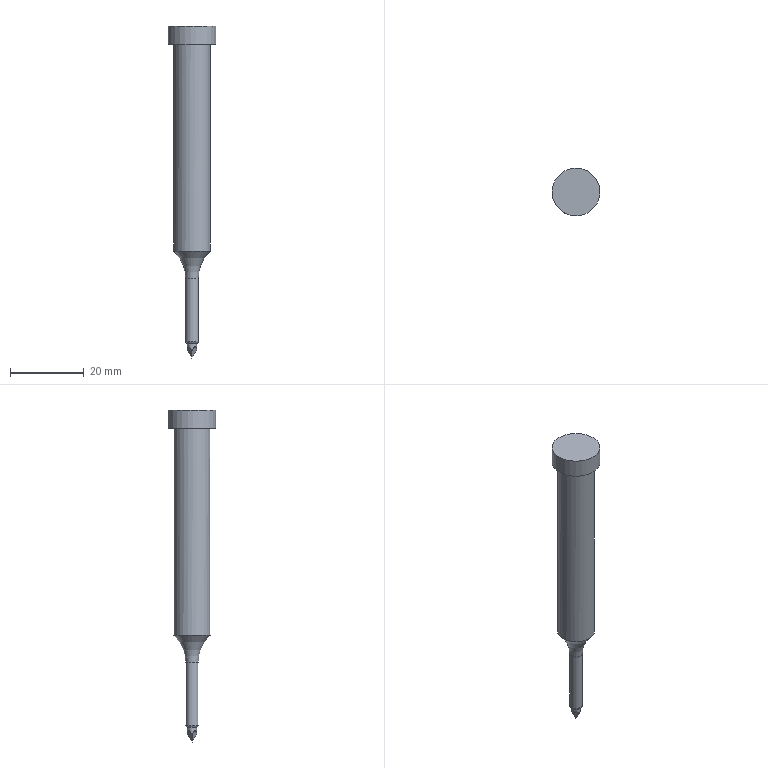Part | NX | features solid 2 | 1 solid | 12 faces | box 13 x 13 x 90 mm | volume 5437 mm3 | plane 6 | cylinder 4 | torus 2 | commonest cylinder face diameters 2.5 x1 3.497 x1 10 x1 13 x1
STEP:
#1=CARTESIAN_POINT('',(78.578,-382.273,-13.5));
#2=VERTEX_POINT('',#1);
#3=CARTESIAN_POINT('',(76.83,-382.273,-13.5));
#4=DIRECTION('',(0.,0.,1.));
#5=DIRECTION('',(1.,0.,0.));
#6=AXIS2_PLACEMENT_3D('',#3,#4,#5);
#7=CIRCLE('',#6,1.748);
#8=EDGE_CURVE('',#2,#2,#7,.F.);
#9=ORIENTED_EDGE('',*,*,#8,.T.);
#10=EDGE_LOOP('',(#9));
#11=FACE_BOUND('',#10,.T.);
#12=CARTESIAN_POINT('',(78.08,-382.273,-14.));
#13=VERTEX_POINT('',#12);
#14=CARTESIAN_POINT('',(76.83,-382.273,-14.));
#15=DIRECTION('',(0.,0.,1.));
#16=DIRECTION('',(1.,0.,0.));
#17=AXIS2_PLACEMENT_3D('',#14,#15,#16);
#18=CIRCLE('',#17,1.25);
#19=EDGE_CURVE('',#13,#13,#18,.T.);
#20=ORIENTED_EDGE('',*,*,#19,.T.);
#21=EDGE_LOOP('',(#20));
#22=FACE_BOUND('',#21,.T.);
#23=CARTESIAN_POINT('',(76.83,-382.273,-13.5));
#24=DIRECTION('',(0.,0.,-1.));
#25=DIRECTION('',(1.,0.,0.));
#26=AXIS2_PLACEMENT_3D('',#23,#24,#25);
#27=TOROIDAL_SURFACE('',#26,1.248,0.5);
#28=ADVANCED_FACE('',(#11,#22),#27,.T.);
#29=CARTESIAN_POINT('',(75.082,-382.273,3.62));
#30=VERTEX_POINT('',#29);
#31=CARTESIAN_POINT('',(76.83,-382.273,3.62));
#32=DIRECTION('',(0.,0.,-1.));
#33=DIRECTION('',(-1.,0.,0.));
#34=AXIS2_PLACEMENT_3D('',#31,#32,#33);
#35=CIRCLE('',#34,1.748);
#36=EDGE_CURVE('',#30,#30,#35,.F.);
#37=ORIENTED_EDGE('',*,*,#36,.F.);
#38=EDGE_LOOP('',(#37));
#39=FACE_BOUND('',#38,.T.);
#40=ORIENTED_EDGE('',*,*,#8,.F.);
#41=EDGE_LOOP('',(#40));
#42=FACE_BOUND('',#41,.T.);
#43=CARTESIAN_POINT('',(76.83,-382.273,-14.));
#44=DIRECTION('',(0.,0.,1.));
#45=DIRECTION('',(-1.,0.,0.));
#46=AXIS2_PLACEMENT_3D('',#43,#44,#45);
#47=CYLINDRICAL_SURFACE('',#46,1.748);
#48=ADVANCED_FACE('',(#39,#42),#47,.T.);
#49=CARTESIAN_POINT('',(81.83,-382.273,11.));
#50=VERTEX_POINT('',#49);
#51=CARTESIAN_POINT('',(76.83,-382.273,11.));
#52=DIRECTION('',(0.,0.,1.));
#53=DIRECTION('',(1.,0.,0.));
#54=AXIS2_PLACEMENT_3D('',#51,#52,#53);
#55=CIRCLE('',#54,5.);
#56=EDGE_CURVE('',#50,#50,#55,.T.);
#57=ORIENTED_EDGE('',*,*,#56,.F.);
#58=EDGE_LOOP('',(#57));
#59=FACE_BOUND('',#58,.T.);
#60=ORIENTED_EDGE('',*,*,#36,.T.);
#61=EDGE_LOOP('',(#60));
#62=FACE_BOUND('',#61,.T.);
#63=CARTESIAN_POINT('',(76.83,-382.273,3.62));
#64=DIRECTION('',(0.,0.,1.));
#65=DIRECTION('',(-1.,0.,0.));
#66=AXIS2_PLACEMENT_3D('',#63,#64,#65);
#67=TOROIDAL_SURFACE('',#66,11.748,10.);
#68=ADVANCED_FACE('',(#59,#62),#67,.F.);
#69=ORIENTED_EDGE('',*,*,#19,.F.);
#70=EDGE_LOOP('',(#69));
#71=FACE_BOUND('',#70,.T.);
#72=CARTESIAN_POINT('',(78.08,-382.273,-15.835));
#73=VERTEX_POINT('',#72);
#74=CARTESIAN_POINT('',(76.83,-383.523,-15.835));
#75=VERTEX_POINT('',#74);
#76=CARTESIAN_POINT('',(76.83,-382.273,-18.));
#77=DIRECTION('',(0.6547,-0.6547,-0.378));
#78=DIRECTION('',(0.2673,-0.2673,0.9258));
#79=AXIS2_PLACEMENT_3D('',#76,#77,#78);
#80=ELLIPSE('',#79,3.307,1.25);
#81=EDGE_CURVE('',#73,#75,#80,.T.);
#82=ORIENTED_EDGE('',*,*,#81,.F.);
#83=CARTESIAN_POINT('',(76.83,-381.023,-15.835));
#84=VERTEX_POINT('',#83);
#85=CARTESIAN_POINT('',(76.83,-382.273,-18.));
#86=DIRECTION('',(0.6547,0.6547,-0.378));
#87=DIRECTION('',(0.2673,0.2673,0.9258));
#88=AXIS2_PLACEMENT_3D('',#85,#86,#87);
#89=ELLIPSE('',#88,3.307,1.25);
#90=EDGE_CURVE('',#84,#73,#89,.T.);
#91=ORIENTED_EDGE('',*,*,#90,.F.);
#92=CARTESIAN_POINT('',(75.58,-382.273,-15.835));
#93=VERTEX_POINT('',#92);
#94=CARTESIAN_POINT('',(76.83,-382.273,-18.));
#95=DIRECTION('',(0.6547,-0.6547,0.378));
#96=DIRECTION('',(-0.2673,0.2673,0.9258));
#97=AXIS2_PLACEMENT_3D('',#94,#95,#96);
#98=ELLIPSE('',#97,3.307,1.25);
#99=EDGE_CURVE('',#84,#93,#98,.T.);
#100=ORIENTED_EDGE('',*,*,#99,.T.);
#101=CARTESIAN_POINT('',(76.83,-382.273,-18.));
#102=DIRECTION('',(-0.6547,-0.6547,-0.378));
#103=DIRECTION('',(-0.2673,-0.2673,0.9258));
#104=AXIS2_PLACEMENT_3D('',#101,#102,#103);
#105=ELLIPSE('',#104,3.307,1.25);
#106=EDGE_CURVE('',#75,#93,#105,.T.);
#107=ORIENTED_EDGE('',*,*,#106,.F.);
#108=EDGE_LOOP('',(#82,#91,#100,#107));
#109=FACE_BOUND('',#108,.T.);
#110=CARTESIAN_POINT('',(76.83,-382.273,-18.));
#111=DIRECTION('',(0.,0.,1.));
#112=DIRECTION('',(-1.,0.,0.));
#113=AXIS2_PLACEMENT_3D('',#110,#111,#112);
#114=CYLINDRICAL_SURFACE('',#113,1.25);
#115=ADVANCED_FACE('',(#71,#109),#114,.T.);
#116=CARTESIAN_POINT('',(76.83,-382.273,-18.));
#117=VERTEX_POINT('',#116);
#118=CARTESIAN_POINT('',(76.83,-382.273,-18.));
#119=DIRECTION('',(0.5,0.,0.866));
#120=VECTOR('',#119,1000.);
#121=LINE('',#118,#120);
#122=EDGE_CURVE('',#73,#117,#121,.F.);
#123=ORIENTED_EDGE('',*,*,#122,.F.);
#124=ORIENTED_EDGE('',*,*,#81,.T.);
#125=CARTESIAN_POINT('',(76.83,-382.273,-18.));
#126=DIRECTION('',(0.,0.5,-0.866));
#127=VECTOR('',#126,1000.);
#128=LINE('',#125,#127);
#129=EDGE_CURVE('',#117,#75,#128,.F.);
#130=ORIENTED_EDGE('',*,*,#129,.F.);
#131=EDGE_LOOP('',(#123,#124,#130));
#132=FACE_BOUND('',#131,.T.);
#133=CARTESIAN_POINT('',(76.83,-382.273,-18.));
#134=DIRECTION('',(-0.6547,0.6547,0.378));
#135=DIRECTION('',(-0.7071,-0.7071,0.));
#136=AXIS2_PLACEMENT_3D('',#133,#134,#135);
#137=PLANE('',#136);
#138=ADVANCED_FACE('',(#132),#137,.F.);
#139=CARTESIAN_POINT('',(76.83,-382.273,-18.));
#140=DIRECTION('',(0.,0.5,0.866));
#141=VECTOR('',#140,1000.);
#142=LINE('',#139,#141);
#143=EDGE_CURVE('',#84,#117,#142,.F.);
#144=ORIENTED_EDGE('',*,*,#143,.F.);
#145=ORIENTED_EDGE('',*,*,#90,.T.);
#146=ORIENTED_EDGE('',*,*,#122,.T.);
#147=EDGE_LOOP('',(#144,#145,#146));
#148=FACE_BOUND('',#147,.T.);
#149=CARTESIAN_POINT('',(76.83,-382.273,-18.));
#150=DIRECTION('',(-0.6547,-0.6547,0.378));
#151=DIRECTION('',(0.7071,-0.7071,0.));
#152=AXIS2_PLACEMENT_3D('',#149,#150,#151);
#153=PLANE('',#152);
#154=ADVANCED_FACE('',(#148),#153,.F.);
#155=ORIENTED_EDGE('',*,*,#143,.T.);
#156=CARTESIAN_POINT('',(76.83,-382.273,-18.));
#157=DIRECTION('',(0.5,0.,-0.866));
#158=VECTOR('',#157,1000.);
#159=LINE('',#156,#158);
#160=EDGE_CURVE('',#117,#93,#159,.F.);
#161=ORIENTED_EDGE('',*,*,#160,.T.);
#162=ORIENTED_EDGE('',*,*,#99,.F.);
#163=EDGE_LOOP('',(#155,#161,#162));
#164=FACE_BOUND('',#163,.T.);
#165=CARTESIAN_POINT('',(76.83,-382.273,-18.));
#166=DIRECTION('',(-0.6547,0.6547,-0.378));
#167=DIRECTION('',(-0.7071,-0.7071,0.));
#168=AXIS2_PLACEMENT_3D('',#165,#166,#167);
#169=PLANE('',#168);
#170=ADVANCED_FACE('',(#164),#169,.T.);
#171=ORIENTED_EDGE('',*,*,#129,.T.);
#172=ORIENTED_EDGE('',*,*,#106,.T.);
#173=ORIENTED_EDGE('',*,*,#160,.F.);
#174=EDGE_LOOP('',(#171,#172,#173));
#175=FACE_BOUND('',#174,.T.);
#176=CARTESIAN_POINT('',(76.83,-382.273,-18.));
#177=DIRECTION('',(0.6547,0.6547,0.378));
#178=DIRECTION('',(-0.7071,0.7071,0.));
#179=AXIS2_PLACEMENT_3D('',#176,#177,#178);
#180=PLANE('',#179);
#181=ADVANCED_FACE('',(#175),#180,.F.);
#182=CARTESIAN_POINT('',(73.294,-385.808,67.));
#183=VERTEX_POINT('',#182);
#184=CARTESIAN_POINT('',(76.83,-382.273,67.));
#185=DIRECTION('',(0.,0.,1.));
#186=DIRECTION('',(-0.7071,-0.7071,0.));
#187=AXIS2_PLACEMENT_3D('',#184,#185,#186);
#188=CIRCLE('',#187,5.);
#189=EDGE_CURVE('',#183,#183,#188,.T.);
#190=ORIENTED_EDGE('',*,*,#189,.F.);
#191=EDGE_LOOP('',(#190));
#192=FACE_BOUND('',#191,.T.);
#193=ORIENTED_EDGE('',*,*,#56,.T.);
#194=EDGE_LOOP('',(#193));
#195=FACE_BOUND('',#194,.T.);
#196=CARTESIAN_POINT('',(76.83,-382.273,72.));
#197=DIRECTION('',(0.,0.,-1.));
#198=DIRECTION('',(0.7071,0.7071,0.));
#199=AXIS2_PLACEMENT_3D('',#196,#197,#198);
#200=CYLINDRICAL_SURFACE('',#199,5.);
#201=ADVANCED_FACE('',(#192,#195),#200,.T.);
#202=CARTESIAN_POINT('',(72.234,-386.869,72.));
#203=VERTEX_POINT('',#202);
#204=CARTESIAN_POINT('',(76.83,-382.273,72.));
#205=DIRECTION('',(0.,0.,1.));
#206=DIRECTION('',(-0.7071,-0.7071,0.));
#207=AXIS2_PLACEMENT_3D('',#204,#205,#206);
#208=CIRCLE('',#207,6.5);
#209=EDGE_CURVE('',#203,#203,#208,.T.);
#210=ORIENTED_EDGE('',*,*,#209,.T.);
#211=EDGE_LOOP('',(#210));
#212=FACE_BOUND('',#211,.T.);
#213=CARTESIAN_POINT('',(76.83,-382.273,72.));
#214=DIRECTION('',(0.,0.,1.));
#215=DIRECTION('',(-0.7071,-0.7071,0.));
#216=AXIS2_PLACEMENT_3D('',#213,#214,#215);
#217=PLANE('',#216);
#218=ADVANCED_FACE('',(#212),#217,.T.);
#219=CARTESIAN_POINT('',(72.234,-386.869,67.));
#220=VERTEX_POINT('',#219);
#221=CARTESIAN_POINT('',(76.83,-382.273,67.));
#222=DIRECTION('',(0.,0.,1.));
#223=DIRECTION('',(-0.7071,-0.7071,0.));
#224=AXIS2_PLACEMENT_3D('',#221,#222,#223);
#225=CIRCLE('',#224,6.5);
#226=EDGE_CURVE('',#220,#220,#225,.T.);
#227=ORIENTED_EDGE('',*,*,#226,.T.);
#228=EDGE_LOOP('',(#227));
#229=FACE_BOUND('',#228,.T.);
#230=ORIENTED_EDGE('',*,*,#209,.F.);
#231=EDGE_LOOP('',(#230));
#232=FACE_BOUND('',#231,.T.);
#233=CARTESIAN_POINT('',(76.83,-382.273,67.));
#234=DIRECTION('',(0.,0.,1.));
#235=DIRECTION('',(-0.7071,-0.7071,0.));
#236=AXIS2_PLACEMENT_3D('',#233,#234,#235);
#237=CYLINDRICAL_SURFACE('',#236,6.5);
#238=ADVANCED_FACE('',(#229,#232),#237,.T.);
#239=ORIENTED_EDGE('',*,*,#226,.F.);
#240=EDGE_LOOP('',(#239));
#241=FACE_BOUND('',#240,.T.);
#242=ORIENTED_EDGE('',*,*,#189,.T.);
#243=EDGE_LOOP('',(#242));
#244=FACE_BOUND('',#243,.T.);
#245=CARTESIAN_POINT('',(76.83,-382.273,67.));
#246=DIRECTION('',(0.,0.,1.));
#247=DIRECTION('',(-0.7071,-0.7071,0.));
#248=AXIS2_PLACEMENT_3D('',#245,#246,#247);
#249=PLANE('',#248);
#250=ADVANCED_FACE('',(#241,#244),#249,.F.);
#251=CLOSED_SHELL('',(#28,#48,#68,#115,#138,#154,#170,#181,#201,#218,#238,#250));
#252=MANIFOLD_SOLID_BREP('',#251);
#253=(LENGTH_UNIT()NAMED_UNIT(*)SI_UNIT(.MILLI.,.METRE.));
#254=UNCERTAINTY_MEASURE_WITH_UNIT(LENGTH_MEASURE(0.00001),#253,'','');
#255=(NAMED_UNIT(*)PLANE_ANGLE_UNIT()SI_UNIT($,.RADIAN.));
#256=(NAMED_UNIT(*)SI_UNIT($,.STERADIAN.)SOLID_ANGLE_UNIT());
#257=(GEOMETRIC_REPRESENTATION_CONTEXT(3)GLOBAL_UNCERTAINTY_ASSIGNED_CONTEXT((#254))GLOBAL_UNIT_ASSIGNED_CONTEXT((#253,#255,#256))REPRESENTATION_CONTEXT('',''));
#258=ADVANCED_BREP_SHAPE_REPRESENTATION('',(#252),#257);